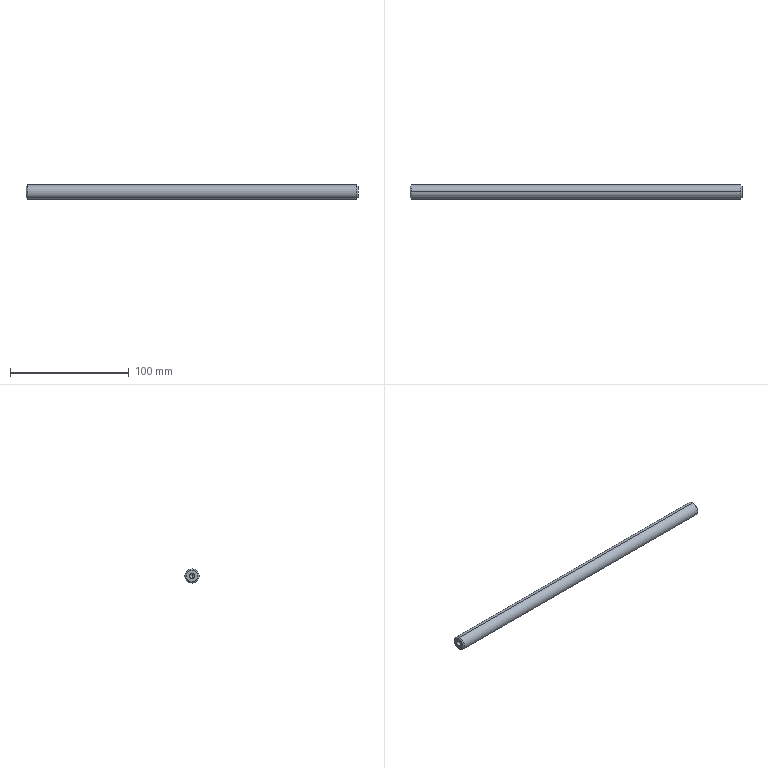Part | STEP file | BPSP-03-016 Lift Chrome Rod_Default | 1 solid | 12 faces | box 280 x 12 x 12 mm | volume 31385 mm3 | cone 6 | cylinder 4 | plane 2 | commonest cylinder face diameters 4.2 x2 12 x2
STEP:
#1=CARTESIAN_POINT('',(0.,0.,0.));
#2=DIRECTION('',(0.,0.,1.));
#3=DIRECTION('',(1.,0.,0.));
#4=AXIS2_PLACEMENT_3D('',#1,#2,#3);
#5=CARTESIAN_POINT('',(17.4,0.,2.1));
#6=VERTEX_POINT('',#5);
#7=CARTESIAN_POINT('',(0.,0.,2.1));
#8=VERTEX_POINT('',#7);
#9=CARTESIAN_POINT('',(0.,0.,2.1));
#10=DIRECTION('',(-1.,0.,0.));
#11=VECTOR('',#10,1.);
#12=LINE('',#9,#11);
#13=CARTESIAN_POINT('',(0.,0.,0.));
#14=DIRECTION('',(-1.,0.,0.));
#15=DIRECTION('',(0.,0.,1.));
#16=AXIS2_PLACEMENT_3D('',#13,#14,#15);
#17=CYLINDRICAL_SURFACE('',#16,2.1);
#18=CARTESIAN_POINT('',(6.283,0.));
#19=DIRECTION('',(0.,1.));
#20=VECTOR('',#19,1.);
#21=LINE('',#18,#20);
#22=(GEOMETRIC_REPRESENTATION_CONTEXT(2)PARAMETRIC_REPRESENTATION_CONTEXT()REPRESENTATION_CONTEXT('',''));
#23=DEFINITIONAL_REPRESENTATION('',(#21),#22);
#24=PCURVE('',#17,#23);
#25=CARTESIAN_POINT('',(0.,0.,0.));
#26=DIRECTION('',(-1.,0.,0.));
#27=DIRECTION('',(0.,0.,1.));
#28=AXIS2_PLACEMENT_3D('',#25,#26,#27);
#29=CYLINDRICAL_SURFACE('',#28,2.1);
#30=CARTESIAN_POINT('',(0.,0.));
#31=DIRECTION('',(0.,1.));
#32=VECTOR('',#31,1.);
#33=LINE('',#30,#32);
#34=(GEOMETRIC_REPRESENTATION_CONTEXT(2)PARAMETRIC_REPRESENTATION_CONTEXT()REPRESENTATION_CONTEXT('',''));
#35=DEFINITIONAL_REPRESENTATION('',(#33),#34);
#36=PCURVE('',#29,#35);
#37=SURFACE_CURVE('',#12,(#24,#36),.PCURVE_S1.);
#38=EDGE_CURVE('',#6,#8,#37,.T.);
#39=ORIENTED_EDGE('',*,*,#38,.T.);
#40=CARTESIAN_POINT('',(0.,0.,-2.1));
#41=VERTEX_POINT('',#40);
#42=CARTESIAN_POINT('',(0.,0.,0.));
#43=DIRECTION('',(-1.,0.,0.));
#44=DIRECTION('',(0.,0.,1.));
#45=AXIS2_PLACEMENT_3D('',#42,#43,#44);
#46=CIRCLE('',#45,2.1);
#47=CARTESIAN_POINT('',(0.,0.));
#48=DIRECTION('',(1.,0.));
#49=VECTOR('',#48,1.);
#50=LINE('',#47,#49);
#51=(GEOMETRIC_REPRESENTATION_CONTEXT(2)PARAMETRIC_REPRESENTATION_CONTEXT()REPRESENTATION_CONTEXT('',''));
#52=DEFINITIONAL_REPRESENTATION('',(#50),#51);
#53=PCURVE('',#17,#52);
#54=CARTESIAN_POINT('',(0.,0.,0.));
#55=DIRECTION('',(1.,0.,0.));
#56=DIRECTION('',(0.,0.,-1.));
#57=AXIS2_PLACEMENT_3D('',#54,#55,#56);
#58=PLANE('',#57);
#59=CARTESIAN_POINT('',(-2.1,0.));
#60=CARTESIAN_POINT('',(-2.1,3.637));
#61=CARTESIAN_POINT('',(1.05,1.819));
#62=CARTESIAN_POINT('',(4.2,0.));
#63=CARTESIAN_POINT('',(1.05,-1.819));
#64=CARTESIAN_POINT('',(-2.1,-3.637));
#65=CARTESIAN_POINT('',(-2.1,0.));
#66=(BOUNDED_CURVE()B_SPLINE_CURVE(2,(#59,#60,#61,#62,#63,#64,#65),.UNSPECIFIED.,.T.,.F.)B_SPLINE_CURVE_WITH_KNOTS((1,2,2,2,2,1),(-2.094,0.,2.094,4.189,6.283,8.378),.UNSPECIFIED.)CURVE()GEOMETRIC_REPRESENTATION_ITEM()RATIONAL_B_SPLINE_CURVE((1.,0.5,1.,0.5,1.,0.5,1.))REPRESENTATION_ITEM(''));
#67=(GEOMETRIC_REPRESENTATION_CONTEXT(2)PARAMETRIC_REPRESENTATION_CONTEXT()REPRESENTATION_CONTEXT('',''));
#68=DEFINITIONAL_REPRESENTATION('',(#66),#67);
#69=PCURVE('',#58,#68);
#70=SURFACE_CURVE('',#46,(#53,#69),.PCURVE_S1.);
#71=EDGE_CURVE('',#41,#8,#70,.T.);
#72=ORIENTED_EDGE('',*,*,#71,.F.);
#73=CARTESIAN_POINT('',(17.4,0.,-2.1));
#74=VERTEX_POINT('',#73);
#75=CARTESIAN_POINT('',(0.,0.,-2.1));
#76=DIRECTION('',(-1.,0.,0.));
#77=VECTOR('',#76,1.);
#78=LINE('',#75,#77);
#79=CARTESIAN_POINT('',(3.142,0.));
#80=DIRECTION('',(0.,1.));
#81=VECTOR('',#80,1.);
#82=LINE('',#79,#81);
#83=(GEOMETRIC_REPRESENTATION_CONTEXT(2)PARAMETRIC_REPRESENTATION_CONTEXT()REPRESENTATION_CONTEXT('',''));
#84=DEFINITIONAL_REPRESENTATION('',(#82),#83);
#85=PCURVE('',#17,#84);
#86=CARTESIAN_POINT('',(3.142,0.));
#87=DIRECTION('',(0.,1.));
#88=VECTOR('',#87,1.);
#89=LINE('',#86,#88);
#90=(GEOMETRIC_REPRESENTATION_CONTEXT(2)PARAMETRIC_REPRESENTATION_CONTEXT()REPRESENTATION_CONTEXT('',''));
#91=DEFINITIONAL_REPRESENTATION('',(#89),#90);
#92=PCURVE('',#29,#91);
#93=SURFACE_CURVE('',#78,(#85,#92),.PCURVE_S1.);
#94=EDGE_CURVE('',#74,#41,#93,.T.);
#95=ORIENTED_EDGE('',*,*,#94,.F.);
#96=CARTESIAN_POINT('',(17.4,0.,0.));
#97=DIRECTION('',(-1.,0.,0.));
#98=DIRECTION('',(0.,0.,1.));
#99=AXIS2_PLACEMENT_3D('',#96,#97,#98);
#100=CIRCLE('',#99,2.1);
#101=CARTESIAN_POINT('',(0.,-17.4));
#102=DIRECTION('',(1.,0.));
#103=VECTOR('',#102,1.);
#104=LINE('',#101,#103);
#105=(GEOMETRIC_REPRESENTATION_CONTEXT(2)PARAMETRIC_REPRESENTATION_CONTEXT()REPRESENTATION_CONTEXT('',''));
#106=DEFINITIONAL_REPRESENTATION('',(#104),#105);
#107=PCURVE('',#17,#106);
#108=CARTESIAN_POINT('',(17.4,0.,0.));
#109=DIRECTION('',(-1.,0.,0.));
#110=DIRECTION('',(0.,0.,1.));
#111=AXIS2_PLACEMENT_3D('',#108,#109,#110);
#112=CONICAL_SURFACE('',#111,2.1,1.03);
#113=CARTESIAN_POINT('',(0.,0.));
#114=DIRECTION('',(1.,0.));
#115=VECTOR('',#114,1.);
#116=LINE('',#113,#115);
#117=(GEOMETRIC_REPRESENTATION_CONTEXT(2)PARAMETRIC_REPRESENTATION_CONTEXT()REPRESENTATION_CONTEXT('',''));
#118=DEFINITIONAL_REPRESENTATION('',(#116),#117);
#119=PCURVE('',#112,#118);
#120=SURFACE_CURVE('',#100,(#107,#119),.PCURVE_S1.);
#121=EDGE_CURVE('',#74,#6,#120,.T.);
#122=ORIENTED_EDGE('',*,*,#121,.T.);
#123=EDGE_LOOP('',(#39,#72,#95,#122));
#124=FACE_BOUND('',#123,.F.);
#125=ADVANCED_FACE('',(#124),#17,.F.);
#126=ORIENTED_EDGE('',*,*,#121,.F.);
#127=CARTESIAN_POINT('',(18.662,0.,0.));
#128=VERTEX_POINT('',#127);
#129=CARTESIAN_POINT('',(17.4,0.,-2.1));
#130=DIRECTION('',(-0.515,0.,-0.8572));
#131=VECTOR('',#130,1.);
#132=LINE('',#129,#131);
#133=CARTESIAN_POINT('',(3.142,0.));
#134=DIRECTION('',(0.,1.));
#135=VECTOR('',#134,1.);
#136=LINE('',#133,#135);
#137=(GEOMETRIC_REPRESENTATION_CONTEXT(2)PARAMETRIC_REPRESENTATION_CONTEXT()REPRESENTATION_CONTEXT('',''));
#138=DEFINITIONAL_REPRESENTATION('',(#136),#137);
#139=PCURVE('',#112,#138);
#140=CARTESIAN_POINT('',(17.4,0.,0.));
#141=DIRECTION('',(-1.,0.,0.));
#142=DIRECTION('',(0.,0.,1.));
#143=AXIS2_PLACEMENT_3D('',#140,#141,#142);
#144=CONICAL_SURFACE('',#143,2.1,1.03);
#145=CARTESIAN_POINT('',(3.142,0.));
#146=DIRECTION('',(0.,1.));
#147=VECTOR('',#146,1.);
#148=LINE('',#145,#147);
#149=(GEOMETRIC_REPRESENTATION_CONTEXT(2)PARAMETRIC_REPRESENTATION_CONTEXT()REPRESENTATION_CONTEXT('',''));
#150=DEFINITIONAL_REPRESENTATION('',(#148),#149);
#151=PCURVE('',#144,#150);
#152=SURFACE_CURVE('',#132,(#139,#151),.PCURVE_S1.);
#153=EDGE_CURVE('',#128,#74,#152,.T.);
#154=ORIENTED_EDGE('',*,*,#153,.F.);
#155=CARTESIAN_POINT('',(17.4,0.,2.1));
#156=DIRECTION('',(-0.515,0.,0.8572));
#157=VECTOR('',#156,1.);
#158=LINE('',#155,#157);
#159=CARTESIAN_POINT('',(6.283,0.));
#160=DIRECTION('',(0.,1.));
#161=VECTOR('',#160,1.);
#162=LINE('',#159,#161);
#163=(GEOMETRIC_REPRESENTATION_CONTEXT(2)PARAMETRIC_REPRESENTATION_CONTEXT()REPRESENTATION_CONTEXT('',''));
#164=DEFINITIONAL_REPRESENTATION('',(#162),#163);
#165=PCURVE('',#112,#164);
#166=CARTESIAN_POINT('',(0.,0.));
#167=DIRECTION('',(0.,1.));
#168=VECTOR('',#167,1.);
#169=LINE('',#166,#168);
#170=(GEOMETRIC_REPRESENTATION_CONTEXT(2)PARAMETRIC_REPRESENTATION_CONTEXT()REPRESENTATION_CONTEXT('',''));
#171=DEFINITIONAL_REPRESENTATION('',(#169),#170);
#172=PCURVE('',#144,#171);
#173=SURFACE_CURVE('',#158,(#165,#172),.PCURVE_S1.);
#174=EDGE_CURVE('',#128,#6,#173,.T.);
#175=ORIENTED_EDGE('',*,*,#174,.T.);
#176=EDGE_LOOP('',(#126,#154,#175));
#177=FACE_BOUND('',#176,.F.);
#178=ADVANCED_FACE('',(#177),#112,.F.);
#179=CARTESIAN_POINT('',(280.,0.,-5.));
#180=VERTEX_POINT('',#179);
#181=CARTESIAN_POINT('',(280.,0.,5.));
#182=VERTEX_POINT('',#181);
#183=CARTESIAN_POINT('',(280.,0.,0.));
#184=DIRECTION('',(1.,0.,0.));
#185=DIRECTION('',(0.,0.,-1.));
#186=AXIS2_PLACEMENT_3D('',#183,#184,#185);
#187=CIRCLE('',#186,5.);
#188=CARTESIAN_POINT('',(280.,0.,0.));
#189=DIRECTION('',(-1.,0.,0.));
#190=DIRECTION('',(0.,0.,1.));
#191=AXIS2_PLACEMENT_3D('',#188,#189,#190);
#192=CONICAL_SURFACE('',#191,5.,0.7854);
#193=CARTESIAN_POINT('',(3.142,0.));
#194=DIRECTION('',(-1.,0.));
#195=VECTOR('',#194,1.);
#196=LINE('',#193,#195);
#197=(GEOMETRIC_REPRESENTATION_CONTEXT(2)PARAMETRIC_REPRESENTATION_CONTEXT()REPRESENTATION_CONTEXT('',''));
#198=DEFINITIONAL_REPRESENTATION('',(#196),#197);
#199=PCURVE('',#192,#198);
#200=CARTESIAN_POINT('',(280.,0.,0.));
#201=DIRECTION('',(1.,0.,0.));
#202=DIRECTION('',(0.,0.,-1.));
#203=AXIS2_PLACEMENT_3D('',#200,#201,#202);
#204=PLANE('',#203);
#205=CARTESIAN_POINT('',(0.,0.));
#206=DIRECTION('',(1.,0.));
#207=AXIS2_PLACEMENT_2D('',#205,#206);
#208=CIRCLE('',#207,5.);
#209=(GEOMETRIC_REPRESENTATION_CONTEXT(2)PARAMETRIC_REPRESENTATION_CONTEXT()REPRESENTATION_CONTEXT('',''));
#210=DEFINITIONAL_REPRESENTATION('',(#208),#209);
#211=PCURVE('',#204,#210);
#212=SURFACE_CURVE('',#187,(#199,#211),.PCURVE_S1.);
#213=EDGE_CURVE('',#180,#182,#212,.T.);
#214=ORIENTED_EDGE('',*,*,#213,.F.);
#215=CARTESIAN_POINT('',(279.,0.,-6.));
#216=VERTEX_POINT('',#215);
#217=CARTESIAN_POINT('',(280.,0.,-5.));
#218=DIRECTION('',(-0.7071,0.,-0.7071));
#219=VECTOR('',#218,1.);
#220=LINE('',#217,#219);
#221=CARTESIAN_POINT('',(3.142,0.));
#222=DIRECTION('',(0.,1.));
#223=VECTOR('',#222,1.);
#224=LINE('',#221,#223);
#225=(GEOMETRIC_REPRESENTATION_CONTEXT(2)PARAMETRIC_REPRESENTATION_CONTEXT()REPRESENTATION_CONTEXT('',''));
#226=DEFINITIONAL_REPRESENTATION('',(#224),#225);
#227=PCURVE('',#192,#226);
#228=CARTESIAN_POINT('',(280.,0.,0.));
#229=DIRECTION('',(-1.,0.,0.));
#230=DIRECTION('',(0.,0.,1.));
#231=AXIS2_PLACEMENT_3D('',#228,#229,#230);
#232=CONICAL_SURFACE('',#231,5.,0.7854);
#233=CARTESIAN_POINT('',(3.142,0.));
#234=DIRECTION('',(0.,1.));
#235=VECTOR('',#234,1.);
#236=LINE('',#233,#235);
#237=(GEOMETRIC_REPRESENTATION_CONTEXT(2)PARAMETRIC_REPRESENTATION_CONTEXT()REPRESENTATION_CONTEXT('',''));
#238=DEFINITIONAL_REPRESENTATION('',(#236),#237);
#239=PCURVE('',#232,#238);
#240=SURFACE_CURVE('',#220,(#227,#239),.PCURVE_S1.);
#241=EDGE_CURVE('',#180,#216,#240,.T.);
#242=ORIENTED_EDGE('',*,*,#241,.T.);
#243=CARTESIAN_POINT('',(279.,0.,6.));
#244=VERTEX_POINT('',#243);
#245=CARTESIAN_POINT('',(279.,0.,0.));
#246=DIRECTION('',(-1.,0.,0.));
#247=DIRECTION('',(0.,0.,-1.));
#248=AXIS2_PLACEMENT_3D('',#245,#246,#247);
#249=CIRCLE('',#248,6.);
#250=CARTESIAN_POINT('',(-3.142,1.));
#251=DIRECTION('',(1.,0.));
#252=VECTOR('',#251,1.);
#253=LINE('',#250,#252);
#254=(GEOMETRIC_REPRESENTATION_CONTEXT(2)PARAMETRIC_REPRESENTATION_CONTEXT()REPRESENTATION_CONTEXT('',''));
#255=DEFINITIONAL_REPRESENTATION('',(#253),#254);
#256=PCURVE('',#192,#255);
#257=CARTESIAN_POINT('',(280.,0.,0.));
#258=DIRECTION('',(-1.,0.,0.));
#259=DIRECTION('',(0.,0.,1.));
#260=AXIS2_PLACEMENT_3D('',#257,#258,#259);
#261=CYLINDRICAL_SURFACE('',#260,6.);
#262=CARTESIAN_POINT('',(-3.142,1.));
#263=DIRECTION('',(1.,0.));
#264=VECTOR('',#263,1.);
#265=LINE('',#262,#264);
#266=(GEOMETRIC_REPRESENTATION_CONTEXT(2)PARAMETRIC_REPRESENTATION_CONTEXT()REPRESENTATION_CONTEXT('',''));
#267=DEFINITIONAL_REPRESENTATION('',(#265),#266);
#268=PCURVE('',#261,#267);
#269=SURFACE_CURVE('',#249,(#256,#268),.PCURVE_S1.);
#270=EDGE_CURVE('',#244,#216,#269,.T.);
#271=ORIENTED_EDGE('',*,*,#270,.F.);
#272=CARTESIAN_POINT('',(280.,0.,5.));
#273=DIRECTION('',(-0.7071,0.,0.7071));
#274=VECTOR('',#273,1.);
#275=LINE('',#272,#274);
#276=CARTESIAN_POINT('',(0.,0.));
#277=DIRECTION('',(0.,1.));
#278=VECTOR('',#277,1.);
#279=LINE('',#276,#278);
#280=(GEOMETRIC_REPRESENTATION_CONTEXT(2)PARAMETRIC_REPRESENTATION_CONTEXT()REPRESENTATION_CONTEXT('',''));
#281=DEFINITIONAL_REPRESENTATION('',(#279),#280);
#282=PCURVE('',#192,#281);
#283=CARTESIAN_POINT('',(6.283,0.));
#284=DIRECTION('',(0.,1.));
#285=VECTOR('',#284,1.);
#286=LINE('',#283,#285);
#287=(GEOMETRIC_REPRESENTATION_CONTEXT(2)PARAMETRIC_REPRESENTATION_CONTEXT()REPRESENTATION_CONTEXT('',''));
#288=DEFINITIONAL_REPRESENTATION('',(#286),#287);
#289=PCURVE('',#232,#288);
#290=SURFACE_CURVE('',#275,(#282,#289),.PCURVE_S1.);
#291=EDGE_CURVE('',#182,#244,#290,.T.);
#292=ORIENTED_EDGE('',*,*,#291,.F.);
#293=EDGE_LOOP('',(#214,#242,#271,#292));
#294=FACE_BOUND('',#293,.T.);
#295=ADVANCED_FACE('',(#294),#192,.T.);
#296=CARTESIAN_POINT('',(0.,0.,5.));
#297=VERTEX_POINT('',#296);
#298=CARTESIAN_POINT('',(0.,0.,-5.));
#299=VERTEX_POINT('',#298);
#300=CARTESIAN_POINT('',(0.,0.,0.));
#301=DIRECTION('',(-1.,0.,0.));
#302=DIRECTION('',(0.,0.,-1.));
#303=AXIS2_PLACEMENT_3D('',#300,#301,#302);
#304=CIRCLE('',#303,5.);
#305=CARTESIAN_POINT('',(1.,0.,0.));
#306=DIRECTION('',(1.,0.,0.));
#307=DIRECTION('',(0.,0.,-1.));
#308=AXIS2_PLACEMENT_3D('',#305,#306,#307);
#309=CONICAL_SURFACE('',#308,6.,0.7854);
#310=CARTESIAN_POINT('',(6.283,-1.));
#311=DIRECTION('',(-1.,0.));
#312=VECTOR('',#311,1.);
#313=LINE('',#310,#312);
#314=(GEOMETRIC_REPRESENTATION_CONTEXT(2)PARAMETRIC_REPRESENTATION_CONTEXT()REPRESENTATION_CONTEXT('',''));
#315=DEFINITIONAL_REPRESENTATION('',(#313),#314);
#316=PCURVE('',#309,#315);
#317=CARTESIAN_POINT('',(5.,0.));
#318=CARTESIAN_POINT('',(5.,-8.66));
#319=CARTESIAN_POINT('',(-2.5,-4.33));
#320=CARTESIAN_POINT('',(-10.,0.));
#321=CARTESIAN_POINT('',(-2.5,4.33));
#322=CARTESIAN_POINT('',(5.,8.66));
#323=CARTESIAN_POINT('',(5.,0.));
#324=(BOUNDED_CURVE()B_SPLINE_CURVE(2,(#317,#318,#319,#320,#321,#322,#323),.UNSPECIFIED.,.T.,.F.)B_SPLINE_CURVE_WITH_KNOTS((1,2,2,2,2,1),(-2.094,0.,2.094,4.189,6.283,8.378),.UNSPECIFIED.)CURVE()GEOMETRIC_REPRESENTATION_ITEM()RATIONAL_B_SPLINE_CURVE((1.,0.5,1.,0.5,1.,0.5,1.))REPRESENTATION_ITEM(''));
#325=(GEOMETRIC_REPRESENTATION_CONTEXT(2)PARAMETRIC_REPRESENTATION_CONTEXT()REPRESENTATION_CONTEXT('',''));
#326=DEFINITIONAL_REPRESENTATION('',(#324),#325);
#327=PCURVE('',#58,#326);
#328=SURFACE_CURVE('',#304,(#316,#327),.PCURVE_S1.);
#329=EDGE_CURVE('',#297,#299,#328,.T.);
#330=ORIENTED_EDGE('',*,*,#329,.F.);
#331=CARTESIAN_POINT('',(1.,0.,6.));
#332=VERTEX_POINT('',#331);
#333=CARTESIAN_POINT('',(1.,0.,6.));
#334=DIRECTION('',(0.7071,0.,0.7071));
#335=VECTOR('',#334,1.);
#336=LINE('',#333,#335);
#337=CARTESIAN_POINT('',(3.142,0.));
#338=DIRECTION('',(0.,1.));
#339=VECTOR('',#338,1.);
#340=LINE('',#337,#339);
#341=(GEOMETRIC_REPRESENTATION_CONTEXT(2)PARAMETRIC_REPRESENTATION_CONTEXT()REPRESENTATION_CONTEXT('',''));
#342=DEFINITIONAL_REPRESENTATION('',(#340),#341);
#343=PCURVE('',#309,#342);
#344=CARTESIAN_POINT('',(1.,0.,0.));
#345=DIRECTION('',(1.,0.,0.));
#346=DIRECTION('',(0.,0.,-1.));
#347=AXIS2_PLACEMENT_3D('',#344,#345,#346);
#348=CONICAL_SURFACE('',#347,6.,0.7854);
#349=CARTESIAN_POINT('',(3.142,0.));
#350=DIRECTION('',(0.,1.));
#351=VECTOR('',#350,1.);
#352=LINE('',#349,#351);
#353=(GEOMETRIC_REPRESENTATION_CONTEXT(2)PARAMETRIC_REPRESENTATION_CONTEXT()REPRESENTATION_CONTEXT('',''));
#354=DEFINITIONAL_REPRESENTATION('',(#352),#353);
#355=PCURVE('',#348,#354);
#356=SURFACE_CURVE('',#336,(#343,#355),.PCURVE_S1.);
#357=EDGE_CURVE('',#297,#332,#356,.T.);
#358=ORIENTED_EDGE('',*,*,#357,.T.);
#359=CARTESIAN_POINT('',(1.,0.,-6.));
#360=VERTEX_POINT('',#359);
#361=CARTESIAN_POINT('',(1.,0.,0.));
#362=DIRECTION('',(1.,0.,0.));
#363=DIRECTION('',(0.,0.,-1.));
#364=AXIS2_PLACEMENT_3D('',#361,#362,#363);
#365=CIRCLE('',#364,6.);
#366=CARTESIAN_POINT('',(0.,0.));
#367=DIRECTION('',(1.,0.));
#368=VECTOR('',#367,1.);
#369=LINE('',#366,#368);
#370=(GEOMETRIC_REPRESENTATION_CONTEXT(2)PARAMETRIC_REPRESENTATION_CONTEXT()REPRESENTATION_CONTEXT('',''));
#371=DEFINITIONAL_REPRESENTATION('',(#369),#370);
#372=PCURVE('',#309,#371);
#373=CARTESIAN_POINT('',(3.142,279.));
#374=DIRECTION('',(-1.,0.));
#375=VECTOR('',#374,1.);
#376=LINE('',#373,#375);
#377=(GEOMETRIC_REPRESENTATION_CONTEXT(2)PARAMETRIC_REPRESENTATION_CONTEXT()REPRESENTATION_CONTEXT('',''));
#378=DEFINITIONAL_REPRESENTATION('',(#376),#377);
#379=PCURVE('',#261,#378);
#380=SURFACE_CURVE('',#365,(#372,#379),.PCURVE_S1.);
#381=EDGE_CURVE('',#360,#332,#380,.T.);
#382=ORIENTED_EDGE('',*,*,#381,.F.);
#383=CARTESIAN_POINT('',(1.,0.,-6.));
#384=DIRECTION('',(0.7071,0.,-0.7071));
#385=VECTOR('',#384,1.);
#386=LINE('',#383,#385);
#387=CARTESIAN_POINT('',(0.,0.));
#388=DIRECTION('',(0.,1.));
#389=VECTOR('',#388,1.);
#390=LINE('',#387,#389);
#391=(GEOMETRIC_REPRESENTATION_CONTEXT(2)PARAMETRIC_REPRESENTATION_CONTEXT()REPRESENTATION_CONTEXT('',''));
#392=DEFINITIONAL_REPRESENTATION('',(#390),#391);
#393=PCURVE('',#309,#392);
#394=CARTESIAN_POINT('',(6.283,0.));
#395=DIRECTION('',(0.,1.));
#396=VECTOR('',#395,1.);
#397=LINE('',#394,#396);
#398=(GEOMETRIC_REPRESENTATION_CONTEXT(2)PARAMETRIC_REPRESENTATION_CONTEXT()REPRESENTATION_CONTEXT('',''));
#399=DEFINITIONAL_REPRESENTATION('',(#397),#398);
#400=PCURVE('',#348,#399);
#401=SURFACE_CURVE('',#386,(#393,#400),.PCURVE_S1.);
#402=EDGE_CURVE('',#299,#360,#401,.T.);
#403=ORIENTED_EDGE('',*,*,#402,.F.);
#404=EDGE_LOOP('',(#330,#358,#382,#403));
#405=FACE_BOUND('',#404,.T.);
#406=ADVANCED_FACE('',(#405),#309,.T.);
#407=ORIENTED_EDGE('',*,*,#270,.T.);
#408=CARTESIAN_POINT('',(280.,0.,-6.));
#409=DIRECTION('',(-1.,0.,0.));
#410=VECTOR('',#409,1.);
#411=LINE('',#408,#410);
#412=CARTESIAN_POINT('',(3.142,0.));
#413=DIRECTION('',(0.,1.));
#414=VECTOR('',#413,1.);
#415=LINE('',#412,#414);
#416=(GEOMETRIC_REPRESENTATION_CONTEXT(2)PARAMETRIC_REPRESENTATION_CONTEXT()REPRESENTATION_CONTEXT('',''));
#417=DEFINITIONAL_REPRESENTATION('',(#415),#416);
#418=PCURVE('',#261,#417);
#419=CARTESIAN_POINT('',(280.,0.,0.));
#420=DIRECTION('',(-1.,0.,0.));
#421=DIRECTION('',(0.,0.,1.));
#422=AXIS2_PLACEMENT_3D('',#419,#420,#421);
#423=CYLINDRICAL_SURFACE('',#422,6.);
#424=CARTESIAN_POINT('',(3.142,0.));
#425=DIRECTION('',(0.,1.));
#426=VECTOR('',#425,1.);
#427=LINE('',#424,#426);
#428=(GEOMETRIC_REPRESENTATION_CONTEXT(2)PARAMETRIC_REPRESENTATION_CONTEXT()REPRESENTATION_CONTEXT('',''));
#429=DEFINITIONAL_REPRESENTATION('',(#427),#428);
#430=PCURVE('',#423,#429);
#431=SURFACE_CURVE('',#411,(#418,#430),.PCURVE_S1.);
#432=EDGE_CURVE('',#216,#360,#431,.T.);
#433=ORIENTED_EDGE('',*,*,#432,.T.);
#434=ORIENTED_EDGE('',*,*,#381,.T.);
#435=CARTESIAN_POINT('',(280.,0.,6.));
#436=DIRECTION('',(-1.,0.,0.));
#437=VECTOR('',#436,1.);
#438=LINE('',#435,#437);
#439=CARTESIAN_POINT('',(0.,0.));
#440=DIRECTION('',(0.,1.));
#441=VECTOR('',#440,1.);
#442=LINE('',#439,#441);
#443=(GEOMETRIC_REPRESENTATION_CONTEXT(2)PARAMETRIC_REPRESENTATION_CONTEXT()REPRESENTATION_CONTEXT('',''));
#444=DEFINITIONAL_REPRESENTATION('',(#442),#443);
#445=PCURVE('',#261,#444);
#446=CARTESIAN_POINT('',(6.283,0.));
#447=DIRECTION('',(0.,1.));
#448=VECTOR('',#447,1.);
#449=LINE('',#446,#448);
#450=(GEOMETRIC_REPRESENTATION_CONTEXT(2)PARAMETRIC_REPRESENTATION_CONTEXT()REPRESENTATION_CONTEXT('',''));
#451=DEFINITIONAL_REPRESENTATION('',(#449),#450);
#452=PCURVE('',#423,#451);
#453=SURFACE_CURVE('',#438,(#445,#452),.PCURVE_S1.);
#454=EDGE_CURVE('',#244,#332,#453,.T.);
#455=ORIENTED_EDGE('',*,*,#454,.F.);
#456=EDGE_LOOP('',(#407,#433,#434,#455));
#457=FACE_BOUND('',#456,.T.);
#458=ADVANCED_FACE('',(#457),#261,.T.);
#459=ORIENTED_EDGE('',*,*,#432,.F.);
#460=CARTESIAN_POINT('',(279.,0.,0.));
#461=DIRECTION('',(-1.,0.,0.));
#462=DIRECTION('',(0.,0.,-1.));
#463=AXIS2_PLACEMENT_3D('',#460,#461,#462);
#464=CIRCLE('',#463,6.);
#465=CARTESIAN_POINT('',(3.142,1.));
#466=DIRECTION('',(1.,0.));
#467=VECTOR('',#466,1.);
#468=LINE('',#465,#467);
#469=(GEOMETRIC_REPRESENTATION_CONTEXT(2)PARAMETRIC_REPRESENTATION_CONTEXT()REPRESENTATION_CONTEXT('',''));
#470=DEFINITIONAL_REPRESENTATION('',(#468),#469);
#471=PCURVE('',#423,#470);
#472=CARTESIAN_POINT('',(3.142,1.));
#473=DIRECTION('',(1.,0.));
#474=VECTOR('',#473,1.);
#475=LINE('',#472,#474);
#476=(GEOMETRIC_REPRESENTATION_CONTEXT(2)PARAMETRIC_REPRESENTATION_CONTEXT()REPRESENTATION_CONTEXT('',''));
#477=DEFINITIONAL_REPRESENTATION('',(#475),#476);
#478=PCURVE('',#232,#477);
#479=SURFACE_CURVE('',#464,(#471,#478),.PCURVE_S1.);
#480=EDGE_CURVE('',#216,#244,#479,.T.);
#481=ORIENTED_EDGE('',*,*,#480,.T.);
#482=ORIENTED_EDGE('',*,*,#454,.T.);
#483=CARTESIAN_POINT('',(1.,0.,0.));
#484=DIRECTION('',(1.,0.,0.));
#485=DIRECTION('',(0.,0.,-1.));
#486=AXIS2_PLACEMENT_3D('',#483,#484,#485);
#487=CIRCLE('',#486,6.);
#488=CARTESIAN_POINT('',(9.425,279.));
#489=DIRECTION('',(-1.,0.));
#490=VECTOR('',#489,1.);
#491=LINE('',#488,#490);
#492=(GEOMETRIC_REPRESENTATION_CONTEXT(2)PARAMETRIC_REPRESENTATION_CONTEXT()REPRESENTATION_CONTEXT('',''));
#493=DEFINITIONAL_REPRESENTATION('',(#491),#492);
#494=PCURVE('',#423,#493);
#495=CARTESIAN_POINT('',(0.,0.));
#496=DIRECTION('',(1.,0.));
#497=VECTOR('',#496,1.);
#498=LINE('',#495,#497);
#499=(GEOMETRIC_REPRESENTATION_CONTEXT(2)PARAMETRIC_REPRESENTATION_CONTEXT()REPRESENTATION_CONTEXT('',''));
#500=DEFINITIONAL_REPRESENTATION('',(#498),#499);
#501=PCURVE('',#348,#500);
#502=SURFACE_CURVE('',#487,(#494,#501),.PCURVE_S1.);
#503=EDGE_CURVE('',#332,#360,#502,.T.);
#504=ORIENTED_EDGE('',*,*,#503,.T.);
#505=EDGE_LOOP('',(#459,#481,#482,#504));
#506=FACE_BOUND('',#505,.T.);
#507=ADVANCED_FACE('',(#506),#423,.T.);
#508=CARTESIAN_POINT('',(280.,0.,0.));
#509=DIRECTION('',(1.,0.,0.));
#510=DIRECTION('',(0.,0.,-1.));
#511=AXIS2_PLACEMENT_3D('',#508,#509,#510);
#512=CIRCLE('',#511,5.);
#513=CARTESIAN_POINT('',(0.,0.));
#514=DIRECTION('',(1.,0.));
#515=AXIS2_PLACEMENT_2D('',#513,#514);
#516=CIRCLE('',#515,5.);
#517=(GEOMETRIC_REPRESENTATION_CONTEXT(2)PARAMETRIC_REPRESENTATION_CONTEXT()REPRESENTATION_CONTEXT('',''));
#518=DEFINITIONAL_REPRESENTATION('',(#516),#517);
#519=PCURVE('',#204,#518);
#520=CARTESIAN_POINT('',(9.425,0.));
#521=DIRECTION('',(-1.,0.));
#522=VECTOR('',#521,1.);
#523=LINE('',#520,#522);
#524=(GEOMETRIC_REPRESENTATION_CONTEXT(2)PARAMETRIC_REPRESENTATION_CONTEXT()REPRESENTATION_CONTEXT('',''));
#525=DEFINITIONAL_REPRESENTATION('',(#523),#524);
#526=PCURVE('',#232,#525);
#527=SURFACE_CURVE('',#512,(#519,#526),.PCURVE_S1.);
#528=EDGE_CURVE('',#182,#180,#527,.T.);
#529=ORIENTED_EDGE('',*,*,#528,.T.);
#530=ORIENTED_EDGE('',*,*,#213,.T.);
#531=EDGE_LOOP('',(#529,#530));
#532=FACE_BOUND('',#531,.T.);
#533=ADVANCED_FACE('',(#532),#204,.T.);
#534=CARTESIAN_POINT('',(0.,0.,0.));
#535=DIRECTION('',(-1.,0.,0.));
#536=DIRECTION('',(0.,0.,1.));
#537=AXIS2_PLACEMENT_3D('',#534,#535,#536);
#538=CIRCLE('',#537,2.1);
#539=CARTESIAN_POINT('',(-2.1,0.));
#540=CARTESIAN_POINT('',(-2.1,3.637));
#541=CARTESIAN_POINT('',(1.05,1.819));
#542=CARTESIAN_POINT('',(4.2,0.));
#543=CARTESIAN_POINT('',(1.05,-1.819));
#544=CARTESIAN_POINT('',(-2.1,-3.637));
#545=CARTESIAN_POINT('',(-2.1,0.));
#546=(BOUNDED_CURVE()B_SPLINE_CURVE(2,(#539,#540,#541,#542,#543,#544,#545),.UNSPECIFIED.,.T.,.F.)B_SPLINE_CURVE_WITH_KNOTS((1,2,2,2,2,1),(-2.094,0.,2.094,4.189,6.283,8.378),.UNSPECIFIED.)CURVE()GEOMETRIC_REPRESENTATION_ITEM()RATIONAL_B_SPLINE_CURVE((1.,0.5,1.,0.5,1.,0.5,1.))REPRESENTATION_ITEM(''));
#547=(GEOMETRIC_REPRESENTATION_CONTEXT(2)PARAMETRIC_REPRESENTATION_CONTEXT()REPRESENTATION_CONTEXT('',''));
#548=DEFINITIONAL_REPRESENTATION('',(#546),#547);
#549=PCURVE('',#58,#548);
#550=CARTESIAN_POINT('',(0.,0.));
#551=DIRECTION('',(1.,0.));
#552=VECTOR('',#551,1.);
#553=LINE('',#550,#552);
#554=(GEOMETRIC_REPRESENTATION_CONTEXT(2)PARAMETRIC_REPRESENTATION_CONTEXT()REPRESENTATION_CONTEXT('',''));
#555=DEFINITIONAL_REPRESENTATION('',(#553),#554);
#556=PCURVE('',#29,#555);
#557=SURFACE_CURVE('',#538,(#549,#556),.PCURVE_S1.);
#558=EDGE_CURVE('',#8,#41,#557,.T.);
#559=ORIENTED_EDGE('',*,*,#558,.F.);
#560=ORIENTED_EDGE('',*,*,#71,.F.);
#561=EDGE_LOOP('',(#559,#560));
#562=FACE_BOUND('',#561,.T.);
#563=CARTESIAN_POINT('',(0.,0.,0.));
#564=DIRECTION('',(-1.,0.,0.));
#565=DIRECTION('',(0.,0.,-1.));
#566=AXIS2_PLACEMENT_3D('',#563,#564,#565);
#567=CIRCLE('',#566,5.);
#568=CARTESIAN_POINT('',(5.,0.));
#569=CARTESIAN_POINT('',(5.,-8.66));
#570=CARTESIAN_POINT('',(-2.5,-4.33));
#571=CARTESIAN_POINT('',(-10.,0.));
#572=CARTESIAN_POINT('',(-2.5,4.33));
#573=CARTESIAN_POINT('',(5.,8.66));
#574=CARTESIAN_POINT('',(5.,0.));
#575=(BOUNDED_CURVE()B_SPLINE_CURVE(2,(#568,#569,#570,#571,#572,#573,#574),.UNSPECIFIED.,.T.,.F.)B_SPLINE_CURVE_WITH_KNOTS((1,2,2,2,2,1),(-2.094,0.,2.094,4.189,6.283,8.378),.UNSPECIFIED.)CURVE()GEOMETRIC_REPRESENTATION_ITEM()RATIONAL_B_SPLINE_CURVE((1.,0.5,1.,0.5,1.,0.5,1.))REPRESENTATION_ITEM(''));
#576=(GEOMETRIC_REPRESENTATION_CONTEXT(2)PARAMETRIC_REPRESENTATION_CONTEXT()REPRESENTATION_CONTEXT('',''));
#577=DEFINITIONAL_REPRESENTATION('',(#575),#576);
#578=PCURVE('',#58,#577);
#579=CARTESIAN_POINT('',(6.283,-1.));
#580=DIRECTION('',(-1.,0.));
#581=VECTOR('',#580,1.);
#582=LINE('',#579,#581);
#583=(GEOMETRIC_REPRESENTATION_CONTEXT(2)PARAMETRIC_REPRESENTATION_CONTEXT()REPRESENTATION_CONTEXT('',''));
#584=DEFINITIONAL_REPRESENTATION('',(#582),#583);
#585=PCURVE('',#348,#584);
#586=SURFACE_CURVE('',#567,(#578,#585),.PCURVE_S1.);
#587=EDGE_CURVE('',#299,#297,#586,.T.);
#588=ORIENTED_EDGE('',*,*,#587,.T.);
#589=ORIENTED_EDGE('',*,*,#329,.T.);
#590=EDGE_LOOP('',(#588,#589));
#591=FACE_BOUND('',#590,.T.);
#592=ADVANCED_FACE('',(#562,#591),#58,.F.);
#593=ORIENTED_EDGE('',*,*,#357,.F.);
#594=ORIENTED_EDGE('',*,*,#587,.F.);
#595=ORIENTED_EDGE('',*,*,#402,.T.);
#596=ORIENTED_EDGE('',*,*,#503,.F.);
#597=EDGE_LOOP('',(#593,#594,#595,#596));
#598=FACE_BOUND('',#597,.T.);
#599=ADVANCED_FACE('',(#598),#348,.T.);
#600=ORIENTED_EDGE('',*,*,#241,.F.);
#601=ORIENTED_EDGE('',*,*,#528,.F.);
#602=ORIENTED_EDGE('',*,*,#291,.T.);
#603=ORIENTED_EDGE('',*,*,#480,.F.);
#604=EDGE_LOOP('',(#600,#601,#602,#603));
#605=FACE_BOUND('',#604,.T.);
#606=ADVANCED_FACE('',(#605),#232,.T.);
#607=CARTESIAN_POINT('',(17.4,0.,0.));
#608=DIRECTION('',(-1.,0.,0.));
#609=DIRECTION('',(0.,0.,1.));
#610=AXIS2_PLACEMENT_3D('',#607,#608,#609);
#611=CIRCLE('',#610,2.1);
#612=CARTESIAN_POINT('',(0.,0.));
#613=DIRECTION('',(1.,0.));
#614=VECTOR('',#613,1.);
#615=LINE('',#612,#614);
#616=(GEOMETRIC_REPRESENTATION_CONTEXT(2)PARAMETRIC_REPRESENTATION_CONTEXT()REPRESENTATION_CONTEXT('',''));
#617=DEFINITIONAL_REPRESENTATION('',(#615),#616);
#618=PCURVE('',#144,#617);
#619=CARTESIAN_POINT('',(0.,-17.4));
#620=DIRECTION('',(1.,0.));
#621=VECTOR('',#620,1.);
#622=LINE('',#619,#621);
#623=(GEOMETRIC_REPRESENTATION_CONTEXT(2)PARAMETRIC_REPRESENTATION_CONTEXT()REPRESENTATION_CONTEXT('',''));
#624=DEFINITIONAL_REPRESENTATION('',(#622),#623);
#625=PCURVE('',#29,#624);
#626=SURFACE_CURVE('',#611,(#618,#625),.PCURVE_S1.);
#627=EDGE_CURVE('',#6,#74,#626,.T.);
#628=ORIENTED_EDGE('',*,*,#627,.F.);
#629=ORIENTED_EDGE('',*,*,#174,.F.);
#630=ORIENTED_EDGE('',*,*,#153,.T.);
#631=EDGE_LOOP('',(#628,#629,#630));
#632=FACE_BOUND('',#631,.F.);
#633=ADVANCED_FACE('',(#632),#144,.F.);
#634=ORIENTED_EDGE('',*,*,#558,.F.);
#635=ORIENTED_EDGE('',*,*,#38,.F.);
#636=ORIENTED_EDGE('',*,*,#627,.T.);
#637=ORIENTED_EDGE('',*,*,#94,.T.);
#638=EDGE_LOOP('',(#634,#635,#636,#637));
#639=FACE_BOUND('',#638,.F.);
#640=ADVANCED_FACE('',(#639),#29,.F.);
#641=CLOSED_SHELL('',(#125,#178,#295,#406,#458,#507,#533,#592,#599,#606,#633,#640));
#642=MANIFOLD_SOLID_BREP('',#641);
#643=(LENGTH_UNIT()NAMED_UNIT(*)SI_UNIT(.MILLI.,.METRE.));
#644=UNCERTAINTY_MEASURE_WITH_UNIT(LENGTH_MEASURE(0.0000001),#643,'','');
#645=(NAMED_UNIT(*)PLANE_ANGLE_UNIT()SI_UNIT($,.RADIAN.));
#646=(NAMED_UNIT(*)SI_UNIT($,.STERADIAN.)SOLID_ANGLE_UNIT());
#647=(GEOMETRIC_REPRESENTATION_CONTEXT(3)GLOBAL_UNCERTAINTY_ASSIGNED_CONTEXT((#644))GLOBAL_UNIT_ASSIGNED_CONTEXT((#643,#645,#646))REPRESENTATION_CONTEXT('',''));
#648=ADVANCED_BREP_SHAPE_REPRESENTATION('',(#4,#642),#647);